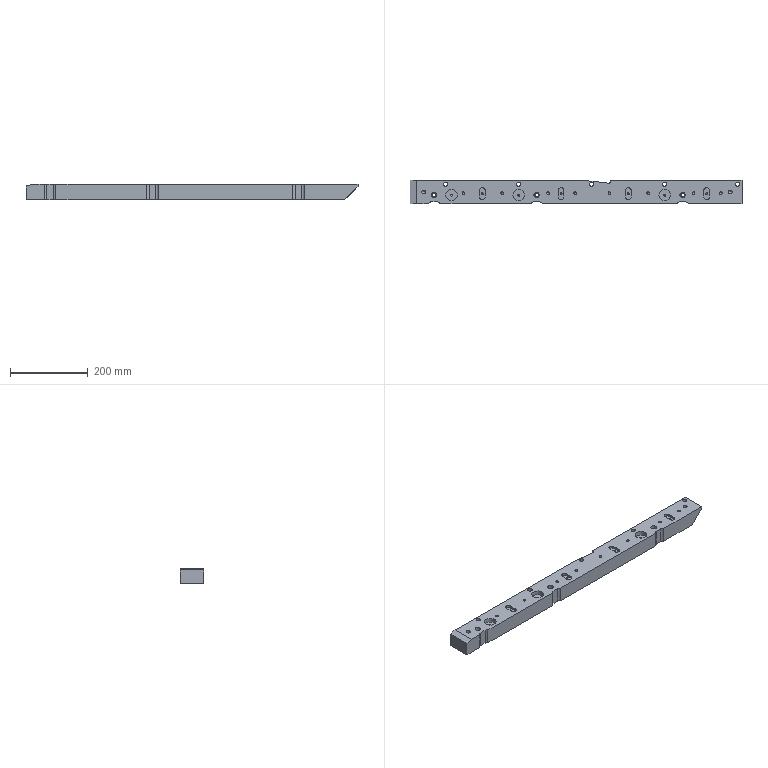Part | NX | features 22 2 | 1 solid | 113 faces | box 855 x 60 x 40 mm | volume 1891796 mm3 | cylinder 55 | plane 41 | cone 17 | commonest cylinder face diameters 14 x9 6.8 x8 15 x8 5.2 x7 6 x6 11 x5